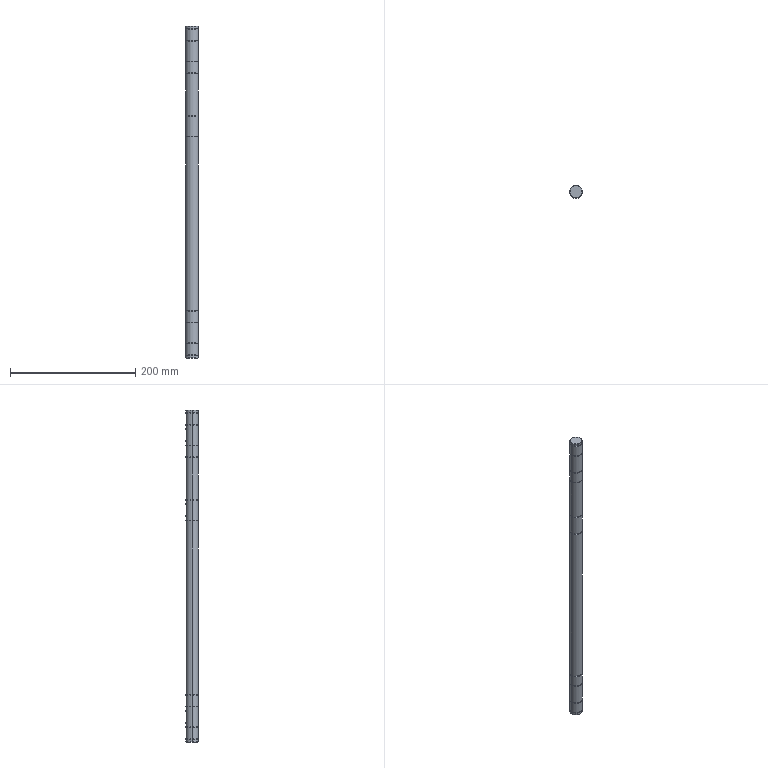Part | STEP file | PN_0014 | 1 solid | 83 faces | box 20 x 20 x 530 mm | volume 164764 mm3 | cylinder 48 | plane 31 | cone 4 | commonest cylinder face diameters 20 x22 18.2 x20 6 x6